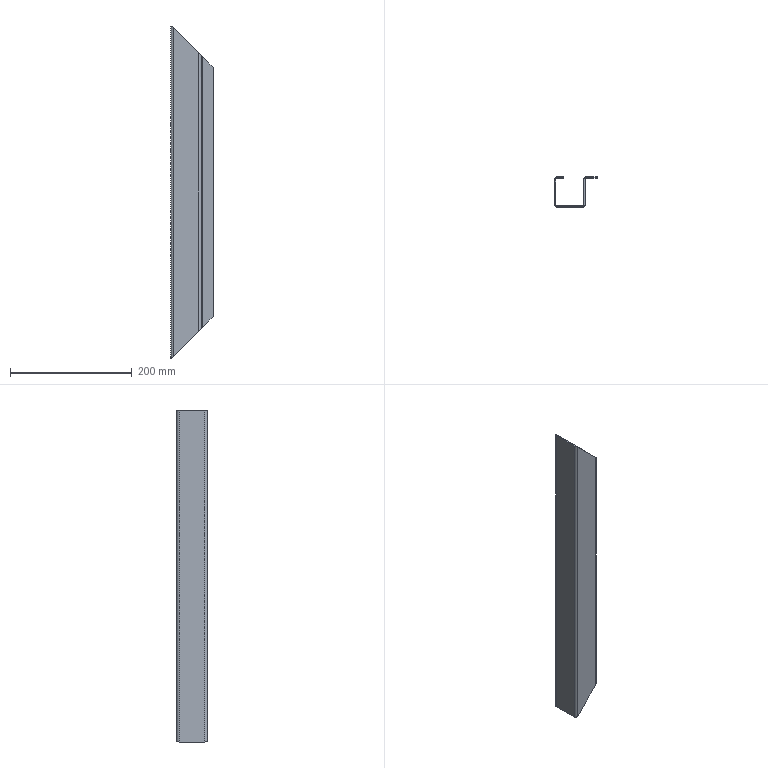Part | STEP file | 750038492 | 1 solid | 38 faces | box 70 x 50 x 546 mm | volume 171514 mm3 | plane 22 | cylinder 8 | spline 8 | commonest cylinder face diameters 4 x4 8 x4
STEP:
#1=CARTESIAN_POINT('',(0.,46.,-273.));
#2=VERTEX_POINT('',#1);
#3=CARTESIAN_POINT('',(0.,4.,-273.));
#4=VERTEX_POINT('',#3);
#5=CARTESIAN_POINT('',(0.,0.,-273.));
#6=DIRECTION('',(0.,-1.,0.));
#7=VECTOR('',#6,1000.);
#8=LINE('',#5,#7);
#9=EDGE_CURVE('',#2,#4,#8,.T.);
#10=ORIENTED_EDGE('',*,*,#9,.T.);
#11=CARTESIAN_POINT('',(0.,4.,273.));
#12=VERTEX_POINT('',#11);
#13=CARTESIAN_POINT('',(0.,4.,275.));
#14=DIRECTION('',(0.,0.,1.));
#15=VECTOR('',#14,1000.);
#16=LINE('',#13,#15);
#17=EDGE_CURVE('',#4,#12,#16,.T.);
#18=ORIENTED_EDGE('',*,*,#17,.T.);
#19=CARTESIAN_POINT('',(0.,46.,273.));
#20=VERTEX_POINT('',#19);
#21=CARTESIAN_POINT('',(0.,0.,273.));
#22=DIRECTION('',(0.,1.,0.));
#23=VECTOR('',#22,1000.);
#24=LINE('',#21,#23);
#25=EDGE_CURVE('',#12,#20,#24,.T.);
#26=ORIENTED_EDGE('',*,*,#25,.T.);
#27=CARTESIAN_POINT('',(0.,46.,275.));
#28=DIRECTION('',(0.,0.,-1.));
#29=VECTOR('',#28,1000.);
#30=LINE('',#27,#29);
#31=EDGE_CURVE('',#20,#2,#30,.T.);
#32=ORIENTED_EDGE('',*,*,#31,.T.);
#33=EDGE_LOOP('',(#10,#18,#26,#32));
#34=FACE_OUTER_BOUND('',#33,.T.);
#35=CARTESIAN_POINT('',(0.,0.,275.));
#36=DIRECTION('',(-1.,0.,0.));
#37=DIRECTION('',(0.,-1.,0.));
#38=AXIS2_PLACEMENT_3D('',#35,#36,#37);
#39=PLANE('',#38);
#40=ADVANCED_FACE('',(#34),#39,.T.);
#41=CARTESIAN_POINT('',(4.,0.,-271.));
#42=VERTEX_POINT('',#41);
#43=CARTESIAN_POINT('',(0.,4.,-273.));
#44=CARTESIAN_POINT('',(0.,2.,-273.));
#45=CARTESIAN_POINT('',(1.333,0.,-272.333));
#46=CARTESIAN_POINT('',(4.,0.,-271.));
#47=(BOUNDED_CURVE()B_SPLINE_CURVE(3,(#43,#44,#45,#46),.UNSPECIFIED.,.F.,.F.)B_SPLINE_CURVE_WITH_KNOTS((4,4),(0.,0.006692),.UNSPECIFIED.)CURVE()GEOMETRIC_REPRESENTATION_ITEM()RATIONAL_B_SPLINE_CURVE((1.,0.6667,0.5,0.5))REPRESENTATION_ITEM(''));
#48=EDGE_CURVE('',#4,#42,#47,.T.);
#49=ORIENTED_EDGE('',*,*,#48,.T.);
#50=CARTESIAN_POINT('',(4.,0.,271.));
#51=VERTEX_POINT('',#50);
#52=CARTESIAN_POINT('',(4.,0.,275.));
#53=DIRECTION('',(0.,0.,1.));
#54=VECTOR('',#53,1000.);
#55=LINE('',#52,#54);
#56=EDGE_CURVE('',#42,#51,#55,.T.);
#57=ORIENTED_EDGE('',*,*,#56,.T.);
#58=CARTESIAN_POINT('',(4.,0.,271.));
#59=CARTESIAN_POINT('',(1.333,0.,272.333));
#60=CARTESIAN_POINT('',(0.,2.,273.));
#61=CARTESIAN_POINT('',(0.,4.,273.));
#62=(BOUNDED_CURVE()B_SPLINE_CURVE(3,(#58,#59,#60,#61),.UNSPECIFIED.,.F.,.F.)B_SPLINE_CURVE_WITH_KNOTS((4,4),(0.,0.006641),.UNSPECIFIED.)CURVE()GEOMETRIC_REPRESENTATION_ITEM()RATIONAL_B_SPLINE_CURVE((0.5,0.5,0.6667,1.))REPRESENTATION_ITEM(''));
#63=EDGE_CURVE('',#51,#12,#62,.T.);
#64=ORIENTED_EDGE('',*,*,#63,.T.);
#65=ORIENTED_EDGE('',*,*,#17,.F.);
#66=EDGE_LOOP('',(#49,#57,#64,#65));
#67=FACE_OUTER_BOUND('',#66,.T.);
#68=CARTESIAN_POINT('',(4.,4.,275.));
#69=DIRECTION('',(0.,0.,-1.));
#70=DIRECTION('',(-1.,0.,0.));
#71=AXIS2_PLACEMENT_3D('',#68,#69,#70);
#72=CYLINDRICAL_SURFACE('',#71,4.);
#73=ADVANCED_FACE('',(#67),#72,.T.);
#74=CARTESIAN_POINT('',(2.,46.,-273.));
#75=VERTEX_POINT('',#74);
#76=CARTESIAN_POINT('',(2.,46.,-273.));
#77=DIRECTION('',(-1.,0.,0.));
#78=VECTOR('',#77,1000.);
#79=LINE('',#76,#78);
#80=EDGE_CURVE('',#75,#2,#79,.T.);
#81=ORIENTED_EDGE('',*,*,#80,.F.);
#82=CARTESIAN_POINT('',(2.,4.,-273.));
#83=VERTEX_POINT('',#82);
#84=CARTESIAN_POINT('',(2.,0.,-273.));
#85=DIRECTION('',(0.,1.,0.));
#86=VECTOR('',#85,1000.);
#87=LINE('',#84,#86);
#88=EDGE_CURVE('',#83,#75,#87,.T.);
#89=ORIENTED_EDGE('',*,*,#88,.F.);
#90=CARTESIAN_POINT('',(2.,4.,-273.));
#91=DIRECTION('',(1.,0.,0.));
#92=VECTOR('',#91,1000.);
#93=LINE('',#90,#92);
#94=EDGE_CURVE('',#4,#83,#93,.T.);
#95=ORIENTED_EDGE('',*,*,#94,.F.);
#96=ORIENTED_EDGE('',*,*,#9,.F.);
#97=EDGE_LOOP('',(#81,#89,#95,#96));
#98=FACE_OUTER_BOUND('',#97,.T.);
#99=CARTESIAN_POINT('',(2.,0.,-273.));
#100=DIRECTION('',(0.,0.,1.));
#101=DIRECTION('',(0.,-1.,0.));
#102=AXIS2_PLACEMENT_3D('',#99,#100,#101);
#103=PLANE('',#102);
#104=ADVANCED_FACE('',(#98),#103,.F.);
#105=CARTESIAN_POINT('',(4.,50.,-271.));
#106=VERTEX_POINT('',#105);
#107=CARTESIAN_POINT('',(4.,50.,-271.));
#108=CARTESIAN_POINT('',(1.333,50.,-272.333));
#109=CARTESIAN_POINT('',(0.,48.,-273.));
#110=CARTESIAN_POINT('',(0.,46.,-273.));
#111=(BOUNDED_CURVE()B_SPLINE_CURVE(3,(#107,#108,#109,#110),.UNSPECIFIED.,.F.,.F.)B_SPLINE_CURVE_WITH_KNOTS((4,4),(0.,0.006641),.UNSPECIFIED.)CURVE()GEOMETRIC_REPRESENTATION_ITEM()RATIONAL_B_SPLINE_CURVE((0.5,0.5,0.6667,1.))REPRESENTATION_ITEM(''));
#112=EDGE_CURVE('',#106,#2,#111,.T.);
#113=ORIENTED_EDGE('',*,*,#112,.T.);
#114=ORIENTED_EDGE('',*,*,#31,.F.);
#115=CARTESIAN_POINT('',(4.,50.,271.));
#116=VERTEX_POINT('',#115);
#117=CARTESIAN_POINT('',(0.,46.,273.));
#118=CARTESIAN_POINT('',(0.,48.,273.));
#119=CARTESIAN_POINT('',(1.333,50.,272.333));
#120=CARTESIAN_POINT('',(4.,50.,271.));
#121=(BOUNDED_CURVE()B_SPLINE_CURVE(3,(#117,#118,#119,#120),.UNSPECIFIED.,.F.,.F.)B_SPLINE_CURVE_WITH_KNOTS((4,4),(0.,0.006627),.UNSPECIFIED.)CURVE()GEOMETRIC_REPRESENTATION_ITEM()RATIONAL_B_SPLINE_CURVE((1.,0.6667,0.5,0.5))REPRESENTATION_ITEM(''));
#122=EDGE_CURVE('',#20,#116,#121,.T.);
#123=ORIENTED_EDGE('',*,*,#122,.T.);
#124=CARTESIAN_POINT('',(4.,50.,275.));
#125=DIRECTION('',(0.,0.,-1.));
#126=VECTOR('',#125,1000.);
#127=LINE('',#124,#126);
#128=EDGE_CURVE('',#116,#106,#127,.T.);
#129=ORIENTED_EDGE('',*,*,#128,.T.);
#130=EDGE_LOOP('',(#113,#114,#123,#129));
#131=FACE_OUTER_BOUND('',#130,.T.);
#132=CARTESIAN_POINT('',(4.,46.,275.));
#133=DIRECTION('',(0.,0.,-1.));
#134=DIRECTION('',(-1.,0.,0.));
#135=AXIS2_PLACEMENT_3D('',#132,#133,#134);
#136=CYLINDRICAL_SURFACE('',#135,4.);
#137=ADVANCED_FACE('',(#131),#136,.T.);
#138=CARTESIAN_POINT('',(2.,46.,273.));
#139=VERTEX_POINT('',#138);
#140=CARTESIAN_POINT('',(2.,4.,273.));
#141=VERTEX_POINT('',#140);
#142=CARTESIAN_POINT('',(2.,0.,273.));
#143=DIRECTION('',(0.,-1.,0.));
#144=VECTOR('',#143,1000.);
#145=LINE('',#142,#144);
#146=EDGE_CURVE('',#139,#141,#145,.T.);
#147=ORIENTED_EDGE('',*,*,#146,.F.);
#148=CARTESIAN_POINT('',(2.,46.,273.));
#149=DIRECTION('',(1.,0.,0.));
#150=VECTOR('',#149,1000.);
#151=LINE('',#148,#150);
#152=EDGE_CURVE('',#20,#139,#151,.T.);
#153=ORIENTED_EDGE('',*,*,#152,.F.);
#154=ORIENTED_EDGE('',*,*,#25,.F.);
#155=CARTESIAN_POINT('',(2.,4.,273.));
#156=DIRECTION('',(-1.,0.,0.));
#157=VECTOR('',#156,1000.);
#158=LINE('',#155,#157);
#159=EDGE_CURVE('',#141,#12,#158,.T.);
#160=ORIENTED_EDGE('',*,*,#159,.F.);
#161=EDGE_LOOP('',(#147,#153,#154,#160));
#162=FACE_OUTER_BOUND('',#161,.T.);
#163=CARTESIAN_POINT('',(2.,0.,273.));
#164=DIRECTION('',(0.,0.,-1.));
#165=DIRECTION('',(0.,1.,0.));
#166=AXIS2_PLACEMENT_3D('',#163,#164,#165);
#167=PLANE('',#166);
#168=ADVANCED_FACE('',(#162),#167,.F.);
#169=CARTESIAN_POINT('',(46.,0.,-229.));
#170=VERTEX_POINT('',#169);
#171=CARTESIAN_POINT('',(4.,0.,-271.));
#172=DIRECTION('',(0.7071,0.,0.7071));
#173=VECTOR('',#172,1000.);
#174=LINE('',#171,#173);
#175=EDGE_CURVE('',#42,#170,#174,.T.);
#176=ORIENTED_EDGE('',*,*,#175,.T.);
#177=CARTESIAN_POINT('',(46.,0.,229.));
#178=VERTEX_POINT('',#177);
#179=CARTESIAN_POINT('',(46.,0.,275.));
#180=DIRECTION('',(0.,0.,1.));
#181=VECTOR('',#180,1000.);
#182=LINE('',#179,#181);
#183=EDGE_CURVE('',#170,#178,#182,.T.);
#184=ORIENTED_EDGE('',*,*,#183,.T.);
#185=CARTESIAN_POINT('',(46.,0.,229.));
#186=DIRECTION('',(-0.7071,0.,0.7071));
#187=VECTOR('',#186,1000.);
#188=LINE('',#185,#187);
#189=EDGE_CURVE('',#178,#51,#188,.T.);
#190=ORIENTED_EDGE('',*,*,#189,.T.);
#191=ORIENTED_EDGE('',*,*,#56,.F.);
#192=EDGE_LOOP('',(#176,#184,#190,#191));
#193=FACE_OUTER_BOUND('',#192,.T.);
#194=CARTESIAN_POINT('',(50.,0.,275.));
#195=DIRECTION('',(0.,-1.,0.));
#196=DIRECTION('',(0.,0.,-1.));
#197=AXIS2_PLACEMENT_3D('',#194,#195,#196);
#198=PLANE('',#197);
#199=ADVANCED_FACE('',(#193),#198,.T.);
#200=CARTESIAN_POINT('',(4.,2.,-271.));
#201=VERTEX_POINT('',#200);
#202=CARTESIAN_POINT('',(4.,1.,-271.));
#203=DIRECTION('',(0.,-1.,0.));
#204=VECTOR('',#203,1000.);
#205=LINE('',#202,#204);
#206=EDGE_CURVE('',#201,#42,#205,.T.);
#207=ORIENTED_EDGE('',*,*,#206,.T.);
#208=ORIENTED_EDGE('',*,*,#48,.F.);
#209=ORIENTED_EDGE('',*,*,#94,.T.);
#210=CARTESIAN_POINT('',(2.,4.,-273.));
#211=CARTESIAN_POINT('',(2.,3.,-273.));
#212=CARTESIAN_POINT('',(2.667,2.,-272.333));
#213=CARTESIAN_POINT('',(4.,2.,-271.));
#214=(BOUNDED_CURVE()B_SPLINE_CURVE(3,(#210,#211,#212,#213),.UNSPECIFIED.,.F.,.F.)B_SPLINE_CURVE_WITH_KNOTS((4,4),(0.,0.003854),.UNSPECIFIED.)CURVE()GEOMETRIC_REPRESENTATION_ITEM()RATIONAL_B_SPLINE_CURVE((1.,0.6667,0.5,0.5))REPRESENTATION_ITEM(''));
#215=EDGE_CURVE('',#83,#201,#214,.T.);
#216=ORIENTED_EDGE('',*,*,#215,.T.);
#217=EDGE_LOOP('',(#207,#208,#209,#216));
#218=FACE_OUTER_BOUND('',#217,.T.);
#219=CARTESIAN_POINT('',(0.,4.,-273.));
#220=CARTESIAN_POINT('',(0.6667,4.,-273.));
#221=CARTESIAN_POINT('',(1.333,4.,-273.));
#222=CARTESIAN_POINT('',(2.,4.,-273.));
#223=CARTESIAN_POINT('',(0.,12.,-273.));
#224=CARTESIAN_POINT('',(0.6667,10.667,-273.));
#225=CARTESIAN_POINT('',(1.333,9.333,-273.));
#226=CARTESIAN_POINT('',(2.,8.,-273.));
#227=CARTESIAN_POINT('',(8.,12.,-269.));
#228=CARTESIAN_POINT('',(7.333,10.667,-269.));
#229=CARTESIAN_POINT('',(6.667,9.333,-269.));
#230=CARTESIAN_POINT('',(6.,8.,-269.));
#231=CARTESIAN_POINT('',(8.,4.,-269.));
#232=CARTESIAN_POINT('',(7.333,4.,-269.));
#233=CARTESIAN_POINT('',(6.667,4.,-269.));
#234=CARTESIAN_POINT('',(6.,4.,-269.));
#235=CARTESIAN_POINT('',(8.,-4.,-269.));
#236=CARTESIAN_POINT('',(7.333,-2.667,-269.));
#237=CARTESIAN_POINT('',(6.667,-1.333,-269.));
#238=CARTESIAN_POINT('',(6.,0.,-269.));
#239=CARTESIAN_POINT('',(0.,-4.,-273.));
#240=CARTESIAN_POINT('',(0.6667,-2.667,-273.));
#241=CARTESIAN_POINT('',(1.333,-1.333,-273.));
#242=CARTESIAN_POINT('',(2.,0.,-273.));
#243=CARTESIAN_POINT('',(0.,4.,-273.));
#244=CARTESIAN_POINT('',(0.6667,4.,-273.));
#245=CARTESIAN_POINT('',(1.333,4.,-273.));
#246=CARTESIAN_POINT('',(2.,4.,-273.));
#247=(BOUNDED_SURFACE()B_SPLINE_SURFACE(3,3,((#219,#220,#221,#222),(#223,#224,#225,#226),(#227,#228,#229,#230),(#231,#232,#233,#234),(#235,#236,#237,#238),(#239,#240,#241,#242),(#243,#244,#245,#246)),.UNSPECIFIED.,.T.,.F.,.F.)B_SPLINE_SURFACE_WITH_KNOTS((4,3,4),(4,4),(0.,0.5,1.),(0.,1.),.UNSPECIFIED.)GEOMETRIC_REPRESENTATION_ITEM()RATIONAL_B_SPLINE_SURFACE(((1.,1.,1.,1.),(0.3333,0.3333,0.3333,0.3333),(0.3333,0.3333,0.3333,0.3333),(1.,1.,1.,1.),(0.3333,0.3333,0.3333,0.3333),(0.3333,0.3333,0.3333,0.3333),(1.,1.,1.,1.)))REPRESENTATION_ITEM('')SURFACE());
#248=ADVANCED_FACE('',(#218),#247,.T.);
#249=ORIENTED_EDGE('',*,*,#159,.T.);
#250=ORIENTED_EDGE('',*,*,#63,.F.);
#251=CARTESIAN_POINT('',(4.,2.,271.));
#252=VERTEX_POINT('',#251);
#253=CARTESIAN_POINT('',(4.,1.,271.));
#254=DIRECTION('',(0.,1.,0.));
#255=VECTOR('',#254,1000.);
#256=LINE('',#253,#255);
#257=EDGE_CURVE('',#51,#252,#256,.T.);
#258=ORIENTED_EDGE('',*,*,#257,.T.);
#259=CARTESIAN_POINT('',(4.,2.,271.));
#260=CARTESIAN_POINT('',(2.667,2.,272.333));
#261=CARTESIAN_POINT('',(2.,3.,273.));
#262=CARTESIAN_POINT('',(2.,4.,273.));
#263=(BOUNDED_CURVE()B_SPLINE_CURVE(3,(#259,#260,#261,#262),.UNSPECIFIED.,.F.,.F.)B_SPLINE_CURVE_WITH_KNOTS((4,4),(0.,0.003785),.UNSPECIFIED.)CURVE()GEOMETRIC_REPRESENTATION_ITEM()RATIONAL_B_SPLINE_CURVE((0.5,0.5,0.6667,1.))REPRESENTATION_ITEM(''));
#264=EDGE_CURVE('',#252,#141,#263,.T.);
#265=ORIENTED_EDGE('',*,*,#264,.T.);
#266=EDGE_LOOP('',(#249,#250,#258,#265));
#267=FACE_OUTER_BOUND('',#266,.T.);
#268=CARTESIAN_POINT('',(8.,4.,269.));
#269=CARTESIAN_POINT('',(7.333,4.,269.));
#270=CARTESIAN_POINT('',(6.667,4.,269.));
#271=CARTESIAN_POINT('',(6.,4.,269.));
#272=CARTESIAN_POINT('',(8.,12.,269.));
#273=CARTESIAN_POINT('',(7.333,10.667,269.));
#274=CARTESIAN_POINT('',(6.667,9.333,269.));
#275=CARTESIAN_POINT('',(6.,8.,269.));
#276=CARTESIAN_POINT('',(0.,12.,273.));
#277=CARTESIAN_POINT('',(0.6667,10.667,273.));
#278=CARTESIAN_POINT('',(1.333,9.333,273.));
#279=CARTESIAN_POINT('',(2.,8.,273.));
#280=CARTESIAN_POINT('',(0.,4.,273.));
#281=CARTESIAN_POINT('',(0.6667,4.,273.));
#282=CARTESIAN_POINT('',(1.333,4.,273.));
#283=CARTESIAN_POINT('',(2.,4.,273.));
#284=CARTESIAN_POINT('',(0.,-4.,273.));
#285=CARTESIAN_POINT('',(0.6667,-2.667,273.));
#286=CARTESIAN_POINT('',(1.333,-1.333,273.));
#287=CARTESIAN_POINT('',(2.,0.,273.));
#288=CARTESIAN_POINT('',(8.,-4.,269.));
#289=CARTESIAN_POINT('',(7.333,-2.667,269.));
#290=CARTESIAN_POINT('',(6.667,-1.333,269.));
#291=CARTESIAN_POINT('',(6.,0.,269.));
#292=CARTESIAN_POINT('',(8.,4.,269.));
#293=CARTESIAN_POINT('',(7.333,4.,269.));
#294=CARTESIAN_POINT('',(6.667,4.,269.));
#295=CARTESIAN_POINT('',(6.,4.,269.));
#296=(BOUNDED_SURFACE()B_SPLINE_SURFACE(3,3,((#268,#269,#270,#271),(#272,#273,#274,#275),(#276,#277,#278,#279),(#280,#281,#282,#283),(#284,#285,#286,#287),(#288,#289,#290,#291),(#292,#293,#294,#295)),.UNSPECIFIED.,.T.,.F.,.F.)B_SPLINE_SURFACE_WITH_KNOTS((4,3,4),(4,4),(0.,0.5,1.),(0.,1.),.UNSPECIFIED.)GEOMETRIC_REPRESENTATION_ITEM()RATIONAL_B_SPLINE_SURFACE(((1.,1.,1.,1.),(0.3333,0.3333,0.3333,0.3333),(0.3333,0.3333,0.3333,0.3333),(1.,1.,1.,1.),(0.3333,0.3333,0.3333,0.3333),(0.3333,0.3333,0.3333,0.3333),(1.,1.,1.,1.)))REPRESENTATION_ITEM('')SURFACE());
#297=ADVANCED_FACE('',(#267),#296,.T.);
#298=ORIENTED_EDGE('',*,*,#80,.T.);
#299=ORIENTED_EDGE('',*,*,#112,.F.);
#300=CARTESIAN_POINT('',(4.,48.,-271.));
#301=VERTEX_POINT('',#300);
#302=CARTESIAN_POINT('',(4.,49.,-271.));
#303=DIRECTION('',(0.,-1.,0.));
#304=VECTOR('',#303,1000.);
#305=LINE('',#302,#304);
#306=EDGE_CURVE('',#106,#301,#305,.T.);
#307=ORIENTED_EDGE('',*,*,#306,.T.);
#308=CARTESIAN_POINT('',(4.,48.,-271.));
#309=CARTESIAN_POINT('',(2.667,48.,-272.333));
#310=CARTESIAN_POINT('',(2.,47.,-273.));
#311=CARTESIAN_POINT('',(2.,46.,-273.));
#312=(BOUNDED_CURVE()B_SPLINE_CURVE(3,(#308,#309,#310,#311),.UNSPECIFIED.,.F.,.F.)B_SPLINE_CURVE_WITH_KNOTS((4,4),(0.,0.003785),.UNSPECIFIED.)CURVE()GEOMETRIC_REPRESENTATION_ITEM()RATIONAL_B_SPLINE_CURVE((0.5,0.5,0.6667,1.))REPRESENTATION_ITEM(''));
#313=EDGE_CURVE('',#301,#75,#312,.T.);
#314=ORIENTED_EDGE('',*,*,#313,.T.);
#315=EDGE_LOOP('',(#298,#299,#307,#314));
#316=FACE_OUTER_BOUND('',#315,.T.);
#317=CARTESIAN_POINT('',(0.,46.,-273.));
#318=CARTESIAN_POINT('',(0.6667,46.,-273.));
#319=CARTESIAN_POINT('',(1.333,46.,-273.));
#320=CARTESIAN_POINT('',(2.,46.,-273.));
#321=CARTESIAN_POINT('',(0.,54.,-273.));
#322=CARTESIAN_POINT('',(0.6667,52.667,-273.));
#323=CARTESIAN_POINT('',(1.333,51.333,-273.));
#324=CARTESIAN_POINT('',(2.,50.,-273.));
#325=CARTESIAN_POINT('',(8.,54.,-269.));
#326=CARTESIAN_POINT('',(7.333,52.667,-269.));
#327=CARTESIAN_POINT('',(6.667,51.333,-269.));
#328=CARTESIAN_POINT('',(6.,50.,-269.));
#329=CARTESIAN_POINT('',(8.,46.,-269.));
#330=CARTESIAN_POINT('',(7.333,46.,-269.));
#331=CARTESIAN_POINT('',(6.667,46.,-269.));
#332=CARTESIAN_POINT('',(6.,46.,-269.));
#333=CARTESIAN_POINT('',(8.,38.,-269.));
#334=CARTESIAN_POINT('',(7.333,39.333,-269.));
#335=CARTESIAN_POINT('',(6.667,40.667,-269.));
#336=CARTESIAN_POINT('',(6.,42.,-269.));
#337=CARTESIAN_POINT('',(0.,38.,-273.));
#338=CARTESIAN_POINT('',(0.6667,39.333,-273.));
#339=CARTESIAN_POINT('',(1.333,40.667,-273.));
#340=CARTESIAN_POINT('',(2.,42.,-273.));
#341=CARTESIAN_POINT('',(0.,46.,-273.));
#342=CARTESIAN_POINT('',(0.6667,46.,-273.));
#343=CARTESIAN_POINT('',(1.333,46.,-273.));
#344=CARTESIAN_POINT('',(2.,46.,-273.));
#345=(BOUNDED_SURFACE()B_SPLINE_SURFACE(3,3,((#317,#318,#319,#320),(#321,#322,#323,#324),(#325,#326,#327,#328),(#329,#330,#331,#332),(#333,#334,#335,#336),(#337,#338,#339,#340),(#341,#342,#343,#344)),.UNSPECIFIED.,.T.,.F.,.F.)B_SPLINE_SURFACE_WITH_KNOTS((4,3,4),(4,4),(0.,0.5,1.),(0.,1.),.UNSPECIFIED.)GEOMETRIC_REPRESENTATION_ITEM()RATIONAL_B_SPLINE_SURFACE(((1.,1.,1.,1.),(0.3333,0.3333,0.3333,0.3333),(0.3333,0.3333,0.3333,0.3333),(1.,1.,1.,1.),(0.3333,0.3333,0.3333,0.3333),(0.3333,0.3333,0.3333,0.3333),(1.,1.,1.,1.)))REPRESENTATION_ITEM('')SURFACE());
#346=ADVANCED_FACE('',(#316),#345,.T.);
#347=ORIENTED_EDGE('',*,*,#146,.T.);
#348=CARTESIAN_POINT('',(2.,4.,275.));
#349=DIRECTION('',(0.,0.,1.));
#350=VECTOR('',#349,1000.);
#351=LINE('',#348,#350);
#352=EDGE_CURVE('',#83,#141,#351,.T.);
#353=ORIENTED_EDGE('',*,*,#352,.F.);
#354=ORIENTED_EDGE('',*,*,#88,.T.);
#355=CARTESIAN_POINT('',(2.,46.,275.));
#356=DIRECTION('',(0.,0.,-1.));
#357=VECTOR('',#356,1000.);
#358=LINE('',#355,#357);
#359=EDGE_CURVE('',#139,#75,#358,.T.);
#360=ORIENTED_EDGE('',*,*,#359,.F.);
#361=EDGE_LOOP('',(#347,#353,#354,#360));
#362=FACE_OUTER_BOUND('',#361,.T.);
#363=CARTESIAN_POINT('',(2.,0.,275.));
#364=DIRECTION('',(-1.,0.,0.));
#365=DIRECTION('',(0.,-1.,0.));
#366=AXIS2_PLACEMENT_3D('',#363,#364,#365);
#367=PLANE('',#366);
#368=ADVANCED_FACE('',(#362),#367,.F.);
#369=CARTESIAN_POINT('',(15.,50.,-260.));
#370=VERTEX_POINT('',#369);
#371=CARTESIAN_POINT('',(15.,50.,-260.));
#372=DIRECTION('',(-0.7071,0.,-0.7071));
#373=VECTOR('',#372,1000.);
#374=LINE('',#371,#373);
#375=EDGE_CURVE('',#370,#106,#374,.T.);
#376=ORIENTED_EDGE('',*,*,#375,.T.);
#377=ORIENTED_EDGE('',*,*,#128,.F.);
#378=CARTESIAN_POINT('',(15.,50.,260.));
#379=VERTEX_POINT('',#378);
#380=CARTESIAN_POINT('',(4.,50.,271.));
#381=DIRECTION('',(0.7071,0.,-0.7071));
#382=VECTOR('',#381,1000.);
#383=LINE('',#380,#382);
#384=EDGE_CURVE('',#116,#379,#383,.T.);
#385=ORIENTED_EDGE('',*,*,#384,.T.);
#386=CARTESIAN_POINT('',(15.,50.,275.));
#387=DIRECTION('',(0.,0.,-1.));
#388=VECTOR('',#387,1000.);
#389=LINE('',#386,#388);
#390=EDGE_CURVE('',#379,#370,#389,.T.);
#391=ORIENTED_EDGE('',*,*,#390,.T.);
#392=EDGE_LOOP('',(#376,#377,#385,#391));
#393=FACE_OUTER_BOUND('',#392,.T.);
#394=CARTESIAN_POINT('',(0.,50.,275.));
#395=DIRECTION('',(0.,1.,0.));
#396=DIRECTION('',(0.,0.,1.));
#397=AXIS2_PLACEMENT_3D('',#394,#395,#396);
#398=PLANE('',#397);
#399=ADVANCED_FACE('',(#393),#398,.T.);
#400=CARTESIAN_POINT('',(4.,48.,271.));
#401=VERTEX_POINT('',#400);
#402=CARTESIAN_POINT('',(4.,49.,271.));
#403=DIRECTION('',(0.,1.,0.));
#404=VECTOR('',#403,1000.);
#405=LINE('',#402,#404);
#406=EDGE_CURVE('',#401,#116,#405,.T.);
#407=ORIENTED_EDGE('',*,*,#406,.T.);
#408=ORIENTED_EDGE('',*,*,#122,.F.);
#409=ORIENTED_EDGE('',*,*,#152,.T.);
#410=CARTESIAN_POINT('',(2.,46.,273.));
#411=CARTESIAN_POINT('',(2.,47.,273.));
#412=CARTESIAN_POINT('',(2.667,48.,272.333));
#413=CARTESIAN_POINT('',(4.,48.,271.));
#414=(BOUNDED_CURVE()B_SPLINE_CURVE(3,(#410,#411,#412,#413),.UNSPECIFIED.,.F.,.F.)B_SPLINE_CURVE_WITH_KNOTS((4,4),(0.,0.003806),.UNSPECIFIED.)CURVE()GEOMETRIC_REPRESENTATION_ITEM()RATIONAL_B_SPLINE_CURVE((1.,0.6667,0.5,0.5))REPRESENTATION_ITEM(''));
#415=EDGE_CURVE('',#139,#401,#414,.T.);
#416=ORIENTED_EDGE('',*,*,#415,.T.);
#417=EDGE_LOOP('',(#407,#408,#409,#416));
#418=FACE_OUTER_BOUND('',#417,.T.);
#419=CARTESIAN_POINT('',(8.,46.,269.));
#420=CARTESIAN_POINT('',(7.333,46.,269.));
#421=CARTESIAN_POINT('',(6.667,46.,269.));
#422=CARTESIAN_POINT('',(6.,46.,269.));
#423=CARTESIAN_POINT('',(8.,54.,269.));
#424=CARTESIAN_POINT('',(7.333,52.667,269.));
#425=CARTESIAN_POINT('',(6.667,51.333,269.));
#426=CARTESIAN_POINT('',(6.,50.,269.));
#427=CARTESIAN_POINT('',(0.,54.,273.));
#428=CARTESIAN_POINT('',(0.6667,52.667,273.));
#429=CARTESIAN_POINT('',(1.333,51.333,273.));
#430=CARTESIAN_POINT('',(2.,50.,273.));
#431=CARTESIAN_POINT('',(0.,46.,273.));
#432=CARTESIAN_POINT('',(0.6667,46.,273.));
#433=CARTESIAN_POINT('',(1.333,46.,273.));
#434=CARTESIAN_POINT('',(2.,46.,273.));
#435=CARTESIAN_POINT('',(0.,38.,273.));
#436=CARTESIAN_POINT('',(0.6667,39.333,273.));
#437=CARTESIAN_POINT('',(1.333,40.667,273.));
#438=CARTESIAN_POINT('',(2.,42.,273.));
#439=CARTESIAN_POINT('',(8.,38.,269.));
#440=CARTESIAN_POINT('',(7.333,39.333,269.));
#441=CARTESIAN_POINT('',(6.667,40.667,269.));
#442=CARTESIAN_POINT('',(6.,42.,269.));
#443=CARTESIAN_POINT('',(8.,46.,269.));
#444=CARTESIAN_POINT('',(7.333,46.,269.));
#445=CARTESIAN_POINT('',(6.667,46.,269.));
#446=CARTESIAN_POINT('',(6.,46.,269.));
#447=(BOUNDED_SURFACE()B_SPLINE_SURFACE(3,3,((#419,#420,#421,#422),(#423,#424,#425,#426),(#427,#428,#429,#430),(#431,#432,#433,#434),(#435,#436,#437,#438),(#439,#440,#441,#442),(#443,#444,#445,#446)),.UNSPECIFIED.,.T.,.F.,.T.)B_SPLINE_SURFACE_WITH_KNOTS((4,3,4),(4,4),(0.,0.5,1.),(0.,1.),.UNSPECIFIED.)GEOMETRIC_REPRESENTATION_ITEM()RATIONAL_B_SPLINE_SURFACE(((1.,1.,1.,1.),(0.3333,0.3333,0.3333,0.3333),(0.3333,0.3333,0.3333,0.3333),(1.,1.,1.,1.),(0.3333,0.3333,0.3333,0.3333),(0.3333,0.3333,0.3333,0.3333),(1.,1.,1.,1.)))REPRESENTATION_ITEM('')SURFACE());
#448=ADVANCED_FACE('',(#418),#447,.T.);
#449=CARTESIAN_POINT('',(50.,4.,-225.));
#450=VERTEX_POINT('',#449);
#451=CARTESIAN_POINT('',(46.,0.,-229.));
#452=CARTESIAN_POINT('',(48.667,0.,-226.333));
#453=CARTESIAN_POINT('',(50.,2.,-225.));
#454=CARTESIAN_POINT('',(50.,4.,-225.));
#455=(BOUNDED_CURVE()B_SPLINE_CURVE(3,(#451,#452,#453,#454),.UNSPECIFIED.,.F.,.T.)B_SPLINE_CURVE_WITH_KNOTS((4,4),(0.,0.007567),.UNSPECIFIED.)CURVE()GEOMETRIC_REPRESENTATION_ITEM()RATIONAL_B_SPLINE_CURVE((0.5,0.5,0.6667,1.))REPRESENTATION_ITEM(''));
#456=EDGE_CURVE('',#170,#450,#455,.T.);
#457=ORIENTED_EDGE('',*,*,#456,.T.);
#458=CARTESIAN_POINT('',(50.,4.,225.));
#459=VERTEX_POINT('',#458);
#460=CARTESIAN_POINT('',(50.,4.,275.));
#461=DIRECTION('',(0.,0.,1.));
#462=VECTOR('',#461,1000.);
#463=LINE('',#460,#462);
#464=EDGE_CURVE('',#450,#459,#463,.T.);
#465=ORIENTED_EDGE('',*,*,#464,.T.);
#466=CARTESIAN_POINT('',(50.,4.,225.));
#467=CARTESIAN_POINT('',(50.,2.,225.));
#468=CARTESIAN_POINT('',(48.667,0.,226.333));
#469=CARTESIAN_POINT('',(46.,0.,229.));
#470=(BOUNDED_CURVE()B_SPLINE_CURVE(3,(#466,#467,#468,#469),.UNSPECIFIED.,.F.,.T.)B_SPLINE_CURVE_WITH_KNOTS((4,4),(0.,0.007712),.UNSPECIFIED.)CURVE()GEOMETRIC_REPRESENTATION_ITEM()RATIONAL_B_SPLINE_CURVE((1.,0.6667,0.5,0.5))REPRESENTATION_ITEM(''));
#471=EDGE_CURVE('',#459,#178,#470,.T.);
#472=ORIENTED_EDGE('',*,*,#471,.T.);
#473=ORIENTED_EDGE('',*,*,#183,.F.);
#474=EDGE_LOOP('',(#457,#465,#472,#473));
#475=FACE_OUTER_BOUND('',#474,.T.);
#476=CARTESIAN_POINT('',(46.,4.,275.));
#477=DIRECTION('',(0.,0.,-1.));
#478=DIRECTION('',(-1.,0.,0.));
#479=AXIS2_PLACEMENT_3D('',#476,#477,#478);
#480=CYLINDRICAL_SURFACE('',#479,4.);
#481=ADVANCED_FACE('',(#475),#480,.T.);
#482=ORIENTED_EDGE('',*,*,#175,.F.);
#483=ORIENTED_EDGE('',*,*,#206,.F.);
#484=CARTESIAN_POINT('',(46.,2.,-229.));
#485=VERTEX_POINT('',#484);
#486=CARTESIAN_POINT('',(300.,2.,25.));
#487=DIRECTION('',(-0.7071,0.,-0.7071));
#488=VECTOR('',#487,1000.);
#489=LINE('',#486,#488);
#490=EDGE_CURVE('',#485,#201,#489,.T.);
#491=ORIENTED_EDGE('',*,*,#490,.F.);
#492=CARTESIAN_POINT('',(46.,0.,-229.));
#493=DIRECTION('',(0.,1.,0.));
#494=VECTOR('',#493,1000.);
#495=LINE('',#492,#494);
#496=EDGE_CURVE('',#170,#485,#495,.T.);
#497=ORIENTED_EDGE('',*,*,#496,.F.);
#498=EDGE_LOOP('',(#482,#483,#491,#497));
#499=FACE_OUTER_BOUND('',#498,.T.);
#500=CARTESIAN_POINT('',(300.,0.,25.));
#501=DIRECTION('',(-0.7071,0.,0.7071));
#502=DIRECTION('',(0.7071,0.,0.7071));
#503=AXIS2_PLACEMENT_3D('',#500,#501,#502);
#504=PLANE('',#503);
#505=ADVANCED_FACE('',(#499),#504,.F.);
#506=ORIENTED_EDGE('',*,*,#189,.F.);
#507=CARTESIAN_POINT('',(46.,2.,229.));
#508=VERTEX_POINT('',#507);
#509=CARTESIAN_POINT('',(46.,0.,229.));
#510=DIRECTION('',(0.,-1.,0.));
#511=VECTOR('',#510,1000.);
#512=LINE('',#509,#511);
#513=EDGE_CURVE('',#508,#178,#512,.T.);
#514=ORIENTED_EDGE('',*,*,#513,.F.);
#515=CARTESIAN_POINT('',(25.,2.,250.));
#516=DIRECTION('',(0.7071,0.,-0.7071));
#517=VECTOR('',#516,1000.);
#518=LINE('',#515,#517);
#519=EDGE_CURVE('',#252,#508,#518,.T.);
#520=ORIENTED_EDGE('',*,*,#519,.F.);
#521=ORIENTED_EDGE('',*,*,#257,.F.);
#522=EDGE_LOOP('',(#506,#514,#520,#521));
#523=FACE_OUTER_BOUND('',#522,.T.);
#524=CARTESIAN_POINT('',(25.,0.,250.));
#525=DIRECTION('',(-0.7071,0.,-0.7071));
#526=DIRECTION('',(-0.7071,0.,0.7071));
#527=AXIS2_PLACEMENT_3D('',#524,#525,#526);
#528=PLANE('',#527);
#529=ADVANCED_FACE('',(#523),#528,.F.);
#530=ORIENTED_EDGE('',*,*,#264,.F.);
#531=CARTESIAN_POINT('',(4.,2.,275.));
#532=DIRECTION('',(0.,0.,1.));
#533=VECTOR('',#532,1000.);
#534=LINE('',#531,#533);
#535=EDGE_CURVE('',#201,#252,#534,.T.);
#536=ORIENTED_EDGE('',*,*,#535,.F.);
#537=ORIENTED_EDGE('',*,*,#215,.F.);
#538=ORIENTED_EDGE('',*,*,#352,.T.);
#539=EDGE_LOOP('',(#530,#536,#537,#538));
#540=FACE_OUTER_BOUND('',#539,.T.);
#541=CARTESIAN_POINT('',(4.,4.,275.));
#542=DIRECTION('',(0.,0.,-1.));
#543=DIRECTION('',(-1.,0.,0.));
#544=AXIS2_PLACEMENT_3D('',#541,#542,#543);
#545=CYLINDRICAL_SURFACE('',#544,2.);
#546=ADVANCED_FACE('',(#540),#545,.F.);
#547=ORIENTED_EDGE('',*,*,#415,.F.);
#548=ORIENTED_EDGE('',*,*,#359,.T.);
#549=ORIENTED_EDGE('',*,*,#313,.F.);
#550=CARTESIAN_POINT('',(4.,48.,275.));
#551=DIRECTION('',(0.,0.,-1.));
#552=VECTOR('',#551,1000.);
#553=LINE('',#550,#552);
#554=EDGE_CURVE('',#401,#301,#553,.T.);
#555=ORIENTED_EDGE('',*,*,#554,.F.);
#556=EDGE_LOOP('',(#547,#548,#549,#555));
#557=FACE_OUTER_BOUND('',#556,.T.);
#558=CARTESIAN_POINT('',(4.,46.,275.));
#559=DIRECTION('',(0.,0.,-1.));
#560=DIRECTION('',(-1.,0.,0.));
#561=AXIS2_PLACEMENT_3D('',#558,#559,#560);
#562=CYLINDRICAL_SURFACE('',#561,2.);
#563=ADVANCED_FACE('',(#557),#562,.F.);
#564=ORIENTED_EDGE('',*,*,#375,.F.);
#565=CARTESIAN_POINT('',(15.,48.,-260.));
#566=VERTEX_POINT('',#565);
#567=CARTESIAN_POINT('',(15.,50.,-260.));
#568=DIRECTION('',(0.,1.,0.));
#569=VECTOR('',#568,1000.);
#570=LINE('',#567,#569);
#571=EDGE_CURVE('',#566,#370,#570,.T.);
#572=ORIENTED_EDGE('',*,*,#571,.F.);
#573=CARTESIAN_POINT('',(275.,48.,0.));
#574=DIRECTION('',(0.7071,0.,0.7071));
#575=VECTOR('',#574,1000.);
#576=LINE('',#573,#575);
#577=EDGE_CURVE('',#301,#566,#576,.T.);
#578=ORIENTED_EDGE('',*,*,#577,.F.);
#579=ORIENTED_EDGE('',*,*,#306,.F.);
#580=EDGE_LOOP('',(#564,#572,#578,#579));
#581=FACE_OUTER_BOUND('',#580,.T.);
#582=CARTESIAN_POINT('',(275.,50.,0.));
#583=DIRECTION('',(-0.7071,0.,0.7071));
#584=DIRECTION('',(0.7071,0.,0.7071));
#585=AXIS2_PLACEMENT_3D('',#582,#583,#584);
#586=PLANE('',#585);
#587=ADVANCED_FACE('',(#581),#586,.F.);
#588=ORIENTED_EDGE('',*,*,#571,.T.);
#589=ORIENTED_EDGE('',*,*,#390,.F.);
#590=CARTESIAN_POINT('',(15.,48.,260.));
#591=VERTEX_POINT('',#590);
#592=CARTESIAN_POINT('',(15.,50.,260.));
#593=DIRECTION('',(0.,-1.,0.));
#594=VECTOR('',#593,1000.);
#595=LINE('',#592,#594);
#596=EDGE_CURVE('',#379,#591,#595,.T.);
#597=ORIENTED_EDGE('',*,*,#596,.T.);
#598=CARTESIAN_POINT('',(15.,48.,275.));
#599=DIRECTION('',(0.,0.,-1.));
#600=VECTOR('',#599,1000.);
#601=LINE('',#598,#600);
#602=EDGE_CURVE('',#591,#566,#601,.T.);
#603=ORIENTED_EDGE('',*,*,#602,.T.);
#604=EDGE_LOOP('',(#588,#589,#597,#603));
#605=FACE_OUTER_BOUND('',#604,.T.);
#606=CARTESIAN_POINT('',(15.,50.,275.));
#607=DIRECTION('',(1.,0.,0.));
#608=DIRECTION('',(0.,0.,-1.));
#609=AXIS2_PLACEMENT_3D('',#606,#607,#608);
#610=PLANE('',#609);
#611=ADVANCED_FACE('',(#605),#610,.T.);
#612=ORIENTED_EDGE('',*,*,#384,.F.);
#613=ORIENTED_EDGE('',*,*,#406,.F.);
#614=CARTESIAN_POINT('',(0.,48.,275.));
#615=DIRECTION('',(-0.7071,0.,0.7071));
#616=VECTOR('',#615,1000.);
#617=LINE('',#614,#616);
#618=EDGE_CURVE('',#591,#401,#617,.T.);
#619=ORIENTED_EDGE('',*,*,#618,.F.);
#620=ORIENTED_EDGE('',*,*,#596,.F.);
#621=EDGE_LOOP('',(#612,#613,#619,#620));
#622=FACE_OUTER_BOUND('',#621,.T.);
#623=CARTESIAN_POINT('',(0.,50.,275.));
#624=DIRECTION('',(-0.7071,0.,-0.7071));
#625=DIRECTION('',(-0.7071,0.,0.7071));
#626=AXIS2_PLACEMENT_3D('',#623,#624,#625);
#627=PLANE('',#626);
#628=ADVANCED_FACE('',(#622),#627,.F.);
#629=CARTESIAN_POINT('',(50.,46.,-225.));
#630=VERTEX_POINT('',#629);
#631=CARTESIAN_POINT('',(50.,48.,-225.));
#632=DIRECTION('',(0.,1.,0.));
#633=VECTOR('',#632,1000.);
#634=LINE('',#631,#633);
#635=EDGE_CURVE('',#450,#630,#634,.T.);
#636=ORIENTED_EDGE('',*,*,#635,.T.);
#637=CARTESIAN_POINT('',(50.,46.,225.));
#638=VERTEX_POINT('',#637);
#639=CARTESIAN_POINT('',(50.,46.,275.));
#640=DIRECTION('',(0.,0.,1.));
#641=VECTOR('',#640,1000.);
#642=LINE('',#639,#641);
#643=EDGE_CURVE('',#630,#638,#642,.T.);
#644=ORIENTED_EDGE('',*,*,#643,.T.);
#645=CARTESIAN_POINT('',(50.,48.,225.));
#646=DIRECTION('',(0.,-1.,0.));
#647=VECTOR('',#646,1000.);
#648=LINE('',#645,#647);
#649=EDGE_CURVE('',#638,#459,#648,.T.);
#650=ORIENTED_EDGE('',*,*,#649,.T.);
#651=ORIENTED_EDGE('',*,*,#464,.F.);
#652=EDGE_LOOP('',(#636,#644,#650,#651));
#653=FACE_OUTER_BOUND('',#652,.T.);
#654=CARTESIAN_POINT('',(50.,48.,275.));
#655=DIRECTION('',(1.,0.,0.));
#656=DIRECTION('',(0.,1.,0.));
#657=AXIS2_PLACEMENT_3D('',#654,#655,#656);
#658=PLANE('',#657);
#659=ADVANCED_FACE('',(#653),#658,.T.);
#660=ORIENTED_EDGE('',*,*,#496,.T.);
#661=CARTESIAN_POINT('',(48.,4.,-225.));
#662=VERTEX_POINT('',#661);
#663=CARTESIAN_POINT('',(46.,2.,-229.));
#664=CARTESIAN_POINT('',(47.333,2.,-226.333));
#665=CARTESIAN_POINT('',(48.,3.,-225.));
#666=CARTESIAN_POINT('',(48.,4.,-225.));
#667=(BOUNDED_CURVE()B_SPLINE_CURVE(3,(#663,#664,#665,#666),.UNSPECIFIED.,.F.,.F.)B_SPLINE_CURVE_WITH_KNOTS((4,4),(0.,0.005228),.UNSPECIFIED.)CURVE()GEOMETRIC_REPRESENTATION_ITEM()RATIONAL_B_SPLINE_CURVE((0.5,0.5,0.6667,1.))REPRESENTATION_ITEM(''));
#668=EDGE_CURVE('',#485,#662,#667,.T.);
#669=ORIENTED_EDGE('',*,*,#668,.T.);
#670=CARTESIAN_POINT('',(49.,4.,-225.));
#671=DIRECTION('',(1.,0.,0.));
#672=VECTOR('',#671,1000.);
#673=LINE('',#670,#672);
#674=EDGE_CURVE('',#662,#450,#673,.T.);
#675=ORIENTED_EDGE('',*,*,#674,.T.);
#676=ORIENTED_EDGE('',*,*,#456,.F.);
#677=EDGE_LOOP('',(#660,#669,#675,#676));
#678=FACE_OUTER_BOUND('',#677,.T.);
#679=CARTESIAN_POINT('',(42.,4.,-233.));
#680=CARTESIAN_POINT('',(42.667,4.,-233.));
#681=CARTESIAN_POINT('',(43.333,4.,-233.));
#682=CARTESIAN_POINT('',(44.,4.,-233.));
#683=CARTESIAN_POINT('',(42.,12.,-233.));
#684=CARTESIAN_POINT('',(42.667,10.667,-233.));
#685=CARTESIAN_POINT('',(43.333,9.333,-233.));
#686=CARTESIAN_POINT('',(44.,8.,-233.));
#687=CARTESIAN_POINT('',(50.,12.,-225.));
#688=CARTESIAN_POINT('',(49.333,10.667,-225.));
#689=CARTESIAN_POINT('',(48.667,9.333,-225.));
#690=CARTESIAN_POINT('',(48.,8.,-225.));
#691=CARTESIAN_POINT('',(50.,4.,-225.));
#692=CARTESIAN_POINT('',(49.333,4.,-225.));
#693=CARTESIAN_POINT('',(48.667,4.,-225.));
#694=CARTESIAN_POINT('',(48.,4.,-225.));
#695=CARTESIAN_POINT('',(50.,-4.,-225.));
#696=CARTESIAN_POINT('',(49.333,-2.667,-225.));
#697=CARTESIAN_POINT('',(48.667,-1.333,-225.));
#698=CARTESIAN_POINT('',(48.,0.,-225.));
#699=CARTESIAN_POINT('',(42.,-4.,-233.));
#700=CARTESIAN_POINT('',(42.667,-2.667,-233.));
#701=CARTESIAN_POINT('',(43.333,-1.333,-233.));
#702=CARTESIAN_POINT('',(44.,0.,-233.));
#703=CARTESIAN_POINT('',(42.,4.,-233.));
#704=CARTESIAN_POINT('',(42.667,4.,-233.));
#705=CARTESIAN_POINT('',(43.333,4.,-233.));
#706=CARTESIAN_POINT('',(44.,4.,-233.));
#707=(BOUNDED_SURFACE()B_SPLINE_SURFACE(3,3,((#679,#680,#681,#682),(#683,#684,#685,#686),(#687,#688,#689,#690),(#691,#692,#693,#694),(#695,#696,#697,#698),(#699,#700,#701,#702),(#703,#704,#705,#706)),.UNSPECIFIED.,.T.,.F.,.T.)B_SPLINE_SURFACE_WITH_KNOTS((4,3,4),(4,4),(0.,0.5,1.),(0.,1.),.UNSPECIFIED.)GEOMETRIC_REPRESENTATION_ITEM()RATIONAL_B_SPLINE_SURFACE(((1.,1.,1.,1.),(0.3333,0.3333,0.3333,0.3333),(0.3333,0.3333,0.3333,0.3333),(1.,1.,1.,1.),(0.3333,0.3333,0.3333,0.3333),(0.3333,0.3333,0.3333,0.3333),(1.,1.,1.,1.)))REPRESENTATION_ITEM('')SURFACE());
#708=ADVANCED_FACE('',(#678),#707,.T.);
#709=CARTESIAN_POINT('',(48.,4.,225.));
#710=VERTEX_POINT('',#709);
#711=CARTESIAN_POINT('',(49.,4.,225.));
#712=DIRECTION('',(-1.,0.,0.));
#713=VECTOR('',#712,1000.);
#714=LINE('',#711,#713);
#715=EDGE_CURVE('',#459,#710,#714,.T.);
#716=ORIENTED_EDGE('',*,*,#715,.T.);
#717=CARTESIAN_POINT('',(48.,4.,225.));
#718=CARTESIAN_POINT('',(48.,3.,225.));
#719=CARTESIAN_POINT('',(47.333,2.,226.333));
#720=CARTESIAN_POINT('',(46.,2.,229.));
#721=(BOUNDED_CURVE()B_SPLINE_CURVE(3,(#717,#718,#719,#720),.UNSPECIFIED.,.F.,.F.)B_SPLINE_CURVE_WITH_KNOTS((4,4),(0.,0.00529),.UNSPECIFIED.)CURVE()GEOMETRIC_REPRESENTATION_ITEM()RATIONAL_B_SPLINE_CURVE((1.,0.6667,0.5,0.5))REPRESENTATION_ITEM(''));
#722=EDGE_CURVE('',#710,#508,#721,.T.);
#723=ORIENTED_EDGE('',*,*,#722,.T.);
#724=ORIENTED_EDGE('',*,*,#513,.T.);
#725=ORIENTED_EDGE('',*,*,#471,.F.);
#726=EDGE_LOOP('',(#716,#723,#724,#725));
#727=FACE_OUTER_BOUND('',#726,.T.);
#728=CARTESIAN_POINT('',(50.,4.,225.));
#729=CARTESIAN_POINT('',(49.333,4.,225.));
#730=CARTESIAN_POINT('',(48.667,4.,225.));
#731=CARTESIAN_POINT('',(48.,4.,225.));
#732=CARTESIAN_POINT('',(50.,12.,225.));
#733=CARTESIAN_POINT('',(49.333,10.667,225.));
#734=CARTESIAN_POINT('',(48.667,9.333,225.));
#735=CARTESIAN_POINT('',(48.,8.,225.));
#736=CARTESIAN_POINT('',(42.,12.,233.));
#737=CARTESIAN_POINT('',(42.667,10.667,233.));
#738=CARTESIAN_POINT('',(43.333,9.333,233.));
#739=CARTESIAN_POINT('',(44.,8.,233.));
#740=CARTESIAN_POINT('',(42.,4.,233.));
#741=CARTESIAN_POINT('',(42.667,4.,233.));
#742=CARTESIAN_POINT('',(43.333,4.,233.));
#743=CARTESIAN_POINT('',(44.,4.,233.));
#744=CARTESIAN_POINT('',(42.,-4.,233.));
#745=CARTESIAN_POINT('',(42.667,-2.667,233.));
#746=CARTESIAN_POINT('',(43.333,-1.333,233.));
#747=CARTESIAN_POINT('',(44.,0.,233.));
#748=CARTESIAN_POINT('',(50.,-4.,225.));
#749=CARTESIAN_POINT('',(49.333,-2.667,225.));
#750=CARTESIAN_POINT('',(48.667,-1.333,225.));
#751=CARTESIAN_POINT('',(48.,0.,225.));
#752=CARTESIAN_POINT('',(50.,4.,225.));
#753=CARTESIAN_POINT('',(49.333,4.,225.));
#754=CARTESIAN_POINT('',(48.667,4.,225.));
#755=CARTESIAN_POINT('',(48.,4.,225.));
#756=(BOUNDED_SURFACE()B_SPLINE_SURFACE(3,3,((#728,#729,#730,#731),(#732,#733,#734,#735),(#736,#737,#738,#739),(#740,#741,#742,#743),(#744,#745,#746,#747),(#748,#749,#750,#751),(#752,#753,#754,#755)),.UNSPECIFIED.,.T.,.F.,.F.)B_SPLINE_SURFACE_WITH_KNOTS((4,3,4),(4,4),(0.,0.5,1.),(0.,1.),.UNSPECIFIED.)GEOMETRIC_REPRESENTATION_ITEM()RATIONAL_B_SPLINE_SURFACE(((1.,1.,1.,1.),(0.3333,0.3333,0.3333,0.3333),(0.3333,0.3333,0.3333,0.3333),(1.,1.,1.,1.),(0.3333,0.3333,0.3333,0.3333),(0.3333,0.3333,0.3333,0.3333),(1.,1.,1.,1.)))REPRESENTATION_ITEM('')SURFACE());
#757=ADVANCED_FACE('',(#727),#756,.T.);
#758=ORIENTED_EDGE('',*,*,#519,.T.);
#759=CARTESIAN_POINT('',(46.,2.,275.));
#760=DIRECTION('',(0.,0.,1.));
#761=VECTOR('',#760,1000.);
#762=LINE('',#759,#761);
#763=EDGE_CURVE('',#485,#508,#762,.T.);
#764=ORIENTED_EDGE('',*,*,#763,.F.);
#765=ORIENTED_EDGE('',*,*,#490,.T.);
#766=ORIENTED_EDGE('',*,*,#535,.T.);
#767=EDGE_LOOP('',(#758,#764,#765,#766));
#768=FACE_OUTER_BOUND('',#767,.T.);
#769=CARTESIAN_POINT('',(50.,2.,275.));
#770=DIRECTION('',(0.,-1.,0.));
#771=DIRECTION('',(0.,0.,-1.));
#772=AXIS2_PLACEMENT_3D('',#769,#770,#771);
#773=PLANE('',#772);
#774=ADVANCED_FACE('',(#768),#773,.F.);
#775=ORIENTED_EDGE('',*,*,#618,.T.);
#776=ORIENTED_EDGE('',*,*,#554,.T.);
#777=ORIENTED_EDGE('',*,*,#577,.T.);
#778=ORIENTED_EDGE('',*,*,#602,.F.);
#779=EDGE_LOOP('',(#775,#776,#777,#778));
#780=FACE_OUTER_BOUND('',#779,.T.);
#781=CARTESIAN_POINT('',(0.,48.,275.));
#782=DIRECTION('',(0.,1.,0.));
#783=DIRECTION('',(0.,0.,1.));
#784=AXIS2_PLACEMENT_3D('',#781,#782,#783);
#785=PLANE('',#784);
#786=ADVANCED_FACE('',(#780),#785,.F.);
#787=ORIENTED_EDGE('',*,*,#643,.F.);
#788=CARTESIAN_POINT('',(52.,48.,-223.));
#789=VERTEX_POINT('',#788);
#790=CARTESIAN_POINT('',(52.,48.,-223.));
#791=CARTESIAN_POINT('',(50.667,48.,-224.333));
#792=CARTESIAN_POINT('',(50.,47.,-225.));
#793=CARTESIAN_POINT('',(50.,46.,-225.));
#794=(BOUNDED_CURVE()B_SPLINE_CURVE(3,(#790,#791,#792,#793),.UNSPECIFIED.,.F.,.F.)B_SPLINE_CURVE_WITH_KNOTS((4,4),(0.,0.003785),.UNSPECIFIED.)CURVE()GEOMETRIC_REPRESENTATION_ITEM()RATIONAL_B_SPLINE_CURVE((0.5,0.5,0.6667,1.))REPRESENTATION_ITEM(''));
#795=EDGE_CURVE('',#789,#630,#794,.T.);
#796=ORIENTED_EDGE('',*,*,#795,.F.);
#797=CARTESIAN_POINT('',(52.,48.,223.));
#798=VERTEX_POINT('',#797);
#799=CARTESIAN_POINT('',(52.,48.,275.));
#800=DIRECTION('',(0.,0.,-1.));
#801=VECTOR('',#800,1000.);
#802=LINE('',#799,#801);
#803=EDGE_CURVE('',#798,#789,#802,.T.);
#804=ORIENTED_EDGE('',*,*,#803,.F.);
#805=CARTESIAN_POINT('',(50.,46.,225.));
#806=CARTESIAN_POINT('',(50.,47.,225.));
#807=CARTESIAN_POINT('',(50.667,48.,224.333));
#808=CARTESIAN_POINT('',(52.,48.,223.));
#809=(BOUNDED_CURVE()B_SPLINE_CURVE(3,(#805,#806,#807,#808),.UNSPECIFIED.,.F.,.F.)B_SPLINE_CURVE_WITH_KNOTS((4,4),(0.,0.003854),.UNSPECIFIED.)CURVE()GEOMETRIC_REPRESENTATION_ITEM()RATIONAL_B_SPLINE_CURVE((1.,0.6667,0.5,0.5))REPRESENTATION_ITEM(''));
#810=EDGE_CURVE('',#638,#798,#809,.T.);
#811=ORIENTED_EDGE('',*,*,#810,.F.);
#812=EDGE_LOOP('',(#787,#796,#804,#811));
#813=FACE_OUTER_BOUND('',#812,.T.);
#814=CARTESIAN_POINT('',(52.,46.,275.));
#815=DIRECTION('',(0.,0.,-1.));
#816=DIRECTION('',(-1.,0.,0.));
#817=AXIS2_PLACEMENT_3D('',#814,#815,#816);
#818=CYLINDRICAL_SURFACE('',#817,2.);
#819=ADVANCED_FACE('',(#813),#818,.F.);
#820=ORIENTED_EDGE('',*,*,#635,.F.);
#821=ORIENTED_EDGE('',*,*,#674,.F.);
#822=CARTESIAN_POINT('',(48.,46.,-225.));
#823=VERTEX_POINT('',#822);
#824=CARTESIAN_POINT('',(48.,48.,-225.));
#825=DIRECTION('',(0.,-1.,0.));
#826=VECTOR('',#825,1000.);
#827=LINE('',#824,#826);
#828=EDGE_CURVE('',#823,#662,#827,.T.);
#829=ORIENTED_EDGE('',*,*,#828,.F.);
#830=CARTESIAN_POINT('',(50.,46.,-225.));
#831=DIRECTION('',(-1.,0.,0.));
#832=VECTOR('',#831,1000.);
#833=LINE('',#830,#832);
#834=EDGE_CURVE('',#630,#823,#833,.T.);
#835=ORIENTED_EDGE('',*,*,#834,.F.);
#836=EDGE_LOOP('',(#820,#821,#829,#835));
#837=FACE_OUTER_BOUND('',#836,.T.);
#838=CARTESIAN_POINT('',(50.,48.,-225.));
#839=DIRECTION('',(0.,0.,1.));
#840=DIRECTION('',(0.,-1.,0.));
#841=AXIS2_PLACEMENT_3D('',#838,#839,#840);
#842=PLANE('',#841);
#843=ADVANCED_FACE('',(#837),#842,.F.);
#844=ORIENTED_EDGE('',*,*,#649,.F.);
#845=CARTESIAN_POINT('',(48.,46.,225.));
#846=VERTEX_POINT('',#845);
#847=CARTESIAN_POINT('',(50.,46.,225.));
#848=DIRECTION('',(1.,0.,0.));
#849=VECTOR('',#848,1000.);
#850=LINE('',#847,#849);
#851=EDGE_CURVE('',#846,#638,#850,.T.);
#852=ORIENTED_EDGE('',*,*,#851,.F.);
#853=CARTESIAN_POINT('',(48.,48.,225.));
#854=DIRECTION('',(0.,1.,0.));
#855=VECTOR('',#854,1000.);
#856=LINE('',#853,#855);
#857=EDGE_CURVE('',#710,#846,#856,.T.);
#858=ORIENTED_EDGE('',*,*,#857,.F.);
#859=ORIENTED_EDGE('',*,*,#715,.F.);
#860=EDGE_LOOP('',(#844,#852,#858,#859));
#861=FACE_OUTER_BOUND('',#860,.T.);
#862=CARTESIAN_POINT('',(50.,48.,225.));
#863=DIRECTION('',(0.,0.,-1.));
#864=DIRECTION('',(0.,1.,0.));
#865=AXIS2_PLACEMENT_3D('',#862,#863,#864);
#866=PLANE('',#865);
#867=ADVANCED_FACE('',(#861),#866,.F.);
#868=ORIENTED_EDGE('',*,*,#722,.F.);
#869=CARTESIAN_POINT('',(48.,4.,275.));
#870=DIRECTION('',(0.,0.,1.));
#871=VECTOR('',#870,1000.);
#872=LINE('',#869,#871);
#873=EDGE_CURVE('',#662,#710,#872,.T.);
#874=ORIENTED_EDGE('',*,*,#873,.F.);
#875=ORIENTED_EDGE('',*,*,#668,.F.);
#876=ORIENTED_EDGE('',*,*,#763,.T.);
#877=EDGE_LOOP('',(#868,#874,#875,#876));
#878=FACE_OUTER_BOUND('',#877,.T.);
#879=CARTESIAN_POINT('',(46.,4.,275.));
#880=DIRECTION('',(0.,0.,-1.));
#881=DIRECTION('',(-1.,0.,0.));
#882=AXIS2_PLACEMENT_3D('',#879,#880,#881);
#883=CYLINDRICAL_SURFACE('',#882,2.);
#884=ADVANCED_FACE('',(#878),#883,.F.);
#885=CARTESIAN_POINT('',(52.,50.,223.));
#886=VERTEX_POINT('',#885);
#887=CARTESIAN_POINT('',(52.,49.,223.));
#888=DIRECTION('',(0.,1.,0.));
#889=VECTOR('',#888,1000.);
#890=LINE('',#887,#889);
#891=EDGE_CURVE('',#798,#886,#890,.T.);
#892=ORIENTED_EDGE('',*,*,#891,.T.);
#893=CARTESIAN_POINT('',(52.,50.,223.));
#894=CARTESIAN_POINT('',(49.333,50.,224.333));
#895=CARTESIAN_POINT('',(48.,48.,225.));
#896=CARTESIAN_POINT('',(48.,46.,225.));
#897=(BOUNDED_CURVE()B_SPLINE_CURVE(3,(#893,#894,#895,#896),.UNSPECIFIED.,.F.,.F.)B_SPLINE_CURVE_WITH_KNOTS((4,4),(0.,0.006622),.UNSPECIFIED.)CURVE()GEOMETRIC_REPRESENTATION_ITEM()RATIONAL_B_SPLINE_CURVE((0.5,0.5,0.6667,1.))REPRESENTATION_ITEM(''));
#898=EDGE_CURVE('',#886,#846,#897,.T.);
#899=ORIENTED_EDGE('',*,*,#898,.T.);
#900=ORIENTED_EDGE('',*,*,#851,.T.);
#901=ORIENTED_EDGE('',*,*,#810,.T.);
#902=EDGE_LOOP('',(#892,#899,#900,#901));
#903=FACE_OUTER_BOUND('',#902,.T.);
#904=CARTESIAN_POINT('',(54.,46.,221.));
#905=CARTESIAN_POINT('',(54.667,46.,221.));
#906=CARTESIAN_POINT('',(55.333,46.,221.));
#907=CARTESIAN_POINT('',(56.,46.,221.));
#908=CARTESIAN_POINT('',(54.,42.,221.));
#909=CARTESIAN_POINT('',(54.667,40.667,221.));
#910=CARTESIAN_POINT('',(55.333,39.333,221.));
#911=CARTESIAN_POINT('',(56.,38.,221.));
#912=CARTESIAN_POINT('',(50.,42.,225.));
#913=CARTESIAN_POINT('',(49.333,40.667,225.));
#914=CARTESIAN_POINT('',(48.667,39.333,225.));
#915=CARTESIAN_POINT('',(48.,38.,225.));
#916=CARTESIAN_POINT('',(50.,46.,225.));
#917=CARTESIAN_POINT('',(49.333,46.,225.));
#918=CARTESIAN_POINT('',(48.667,46.,225.));
#919=CARTESIAN_POINT('',(48.,46.,225.));
#920=CARTESIAN_POINT('',(50.,50.,225.));
#921=CARTESIAN_POINT('',(49.333,51.333,225.));
#922=CARTESIAN_POINT('',(48.667,52.667,225.));
#923=CARTESIAN_POINT('',(48.,54.,225.));
#924=CARTESIAN_POINT('',(54.,50.,221.));
#925=CARTESIAN_POINT('',(54.667,51.333,221.));
#926=CARTESIAN_POINT('',(55.333,52.667,221.));
#927=CARTESIAN_POINT('',(56.,54.,221.));
#928=CARTESIAN_POINT('',(54.,46.,221.));
#929=CARTESIAN_POINT('',(54.667,46.,221.));
#930=CARTESIAN_POINT('',(55.333,46.,221.));
#931=CARTESIAN_POINT('',(56.,46.,221.));
#932=(BOUNDED_SURFACE()B_SPLINE_SURFACE(3,3,((#904,#905,#906,#907),(#908,#909,#910,#911),(#912,#913,#914,#915),(#916,#917,#918,#919),(#920,#921,#922,#923),(#924,#925,#926,#927),(#928,#929,#930,#931)),.UNSPECIFIED.,.T.,.F.,.F.)B_SPLINE_SURFACE_WITH_KNOTS((4,3,4),(4,4),(0.,0.5,1.),(0.,1.),.UNSPECIFIED.)GEOMETRIC_REPRESENTATION_ITEM()RATIONAL_B_SPLINE_SURFACE(((1.,1.,1.,1.),(0.3333,0.3333,0.3333,0.3333),(0.3333,0.3333,0.3333,0.3333),(1.,1.,1.,1.),(0.3333,0.3333,0.3333,0.3333),(0.3333,0.3333,0.3333,0.3333),(1.,1.,1.,1.)))REPRESENTATION_ITEM('')SURFACE());
#933=ADVANCED_FACE('',(#903),#932,.T.);
#934=ORIENTED_EDGE('',*,*,#834,.T.);
#935=CARTESIAN_POINT('',(52.,50.,-223.));
#936=VERTEX_POINT('',#935);
#937=CARTESIAN_POINT('',(48.,46.,-225.));
#938=CARTESIAN_POINT('',(48.,48.,-225.));
#939=CARTESIAN_POINT('',(49.333,50.,-224.333));
#940=CARTESIAN_POINT('',(52.,50.,-223.));
#941=(BOUNDED_CURVE()B_SPLINE_CURVE(3,(#937,#938,#939,#940),.UNSPECIFIED.,.F.,.F.)B_SPLINE_CURVE_WITH_KNOTS((4,4),(0.,0.006696),.UNSPECIFIED.)CURVE()GEOMETRIC_REPRESENTATION_ITEM()RATIONAL_B_SPLINE_CURVE((1.,0.6667,0.5,0.5))REPRESENTATION_ITEM(''));
#942=EDGE_CURVE('',#823,#936,#941,.T.);
#943=ORIENTED_EDGE('',*,*,#942,.T.);
#944=CARTESIAN_POINT('',(52.,49.,-223.));
#945=DIRECTION('',(0.,-1.,0.));
#946=VECTOR('',#945,1000.);
#947=LINE('',#944,#946);
#948=EDGE_CURVE('',#936,#789,#947,.T.);
#949=ORIENTED_EDGE('',*,*,#948,.T.);
#950=ORIENTED_EDGE('',*,*,#795,.T.);
#951=EDGE_LOOP('',(#934,#943,#949,#950));
#952=FACE_OUTER_BOUND('',#951,.T.);
#953=CARTESIAN_POINT('',(50.,46.,-225.));
#954=CARTESIAN_POINT('',(49.333,46.,-225.));
#955=CARTESIAN_POINT('',(48.667,46.,-225.));
#956=CARTESIAN_POINT('',(48.,46.,-225.));
#957=CARTESIAN_POINT('',(50.,42.,-225.));
#958=CARTESIAN_POINT('',(49.333,40.667,-225.));
#959=CARTESIAN_POINT('',(48.667,39.333,-225.));
#960=CARTESIAN_POINT('',(48.,38.,-225.));
#961=CARTESIAN_POINT('',(54.,42.,-221.));
#962=CARTESIAN_POINT('',(54.667,40.667,-221.));
#963=CARTESIAN_POINT('',(55.333,39.333,-221.));
#964=CARTESIAN_POINT('',(56.,38.,-221.));
#965=CARTESIAN_POINT('',(54.,46.,-221.));
#966=CARTESIAN_POINT('',(54.667,46.,-221.));
#967=CARTESIAN_POINT('',(55.333,46.,-221.));
#968=CARTESIAN_POINT('',(56.,46.,-221.));
#969=CARTESIAN_POINT('',(54.,50.,-221.));
#970=CARTESIAN_POINT('',(54.667,51.333,-221.));
#971=CARTESIAN_POINT('',(55.333,52.667,-221.));
#972=CARTESIAN_POINT('',(56.,54.,-221.));
#973=CARTESIAN_POINT('',(50.,50.,-225.));
#974=CARTESIAN_POINT('',(49.333,51.333,-225.));
#975=CARTESIAN_POINT('',(48.667,52.667,-225.));
#976=CARTESIAN_POINT('',(48.,54.,-225.));
#977=CARTESIAN_POINT('',(50.,46.,-225.));
#978=CARTESIAN_POINT('',(49.333,46.,-225.));
#979=CARTESIAN_POINT('',(48.667,46.,-225.));
#980=CARTESIAN_POINT('',(48.,46.,-225.));
#981=(BOUNDED_SURFACE()B_SPLINE_SURFACE(3,3,((#953,#954,#955,#956),(#957,#958,#959,#960),(#961,#962,#963,#964),(#965,#966,#967,#968),(#969,#970,#971,#972),(#973,#974,#975,#976),(#977,#978,#979,#980)),.UNSPECIFIED.,.T.,.F.,.F.)B_SPLINE_SURFACE_WITH_KNOTS((4,3,4),(4,4),(0.,0.5,1.),(0.,1.),.UNSPECIFIED.)GEOMETRIC_REPRESENTATION_ITEM()RATIONAL_B_SPLINE_SURFACE(((1.,1.,1.,1.),(0.3333,0.3333,0.3333,0.3333),(0.3333,0.3333,0.3333,0.3333),(1.,1.,1.,1.),(0.3333,0.3333,0.3333,0.3333),(0.3333,0.3333,0.3333,0.3333),(1.,1.,1.,1.)))REPRESENTATION_ITEM('')SURFACE());
#982=ADVANCED_FACE('',(#952),#981,.T.);
#983=CARTESIAN_POINT('',(70.,48.,-205.));
#984=VERTEX_POINT('',#983);
#985=CARTESIAN_POINT('',(52.,48.,-223.));
#986=DIRECTION('',(0.7071,0.,0.7071));
#987=VECTOR('',#986,1000.);
#988=LINE('',#985,#987);
#989=EDGE_CURVE('',#789,#984,#988,.T.);
#990=ORIENTED_EDGE('',*,*,#989,.T.);
#991=CARTESIAN_POINT('',(70.,48.,205.));
#992=VERTEX_POINT('',#991);
#993=CARTESIAN_POINT('',(70.,48.,275.));
#994=DIRECTION('',(0.,0.,1.));
#995=VECTOR('',#994,1000.);
#996=LINE('',#993,#995);
#997=EDGE_CURVE('',#984,#992,#996,.T.);
#998=ORIENTED_EDGE('',*,*,#997,.T.);
#999=CARTESIAN_POINT('',(70.,48.,205.));
#1000=DIRECTION('',(-0.7071,0.,0.7071));
#1001=VECTOR('',#1000,1000.);
#1002=LINE('',#999,#1001);
#1003=EDGE_CURVE('',#992,#798,#1002,.T.);
#1004=ORIENTED_EDGE('',*,*,#1003,.T.);
#1005=ORIENTED_EDGE('',*,*,#803,.T.);
#1006=EDGE_LOOP('',(#990,#998,#1004,#1005));
#1007=FACE_OUTER_BOUND('',#1006,.T.);
#1008=CARTESIAN_POINT('',(70.,48.,275.));
#1009=DIRECTION('',(0.,-1.,0.));
#1010=DIRECTION('',(0.,0.,-1.));
#1011=AXIS2_PLACEMENT_3D('',#1008,#1009,#1010);
#1012=PLANE('',#1011);
#1013=ADVANCED_FACE('',(#1007),#1012,.T.);
#1014=ORIENTED_EDGE('',*,*,#857,.T.);
#1015=CARTESIAN_POINT('',(48.,46.,275.));
#1016=DIRECTION('',(0.,0.,1.));
#1017=VECTOR('',#1016,1000.);
#1018=LINE('',#1015,#1017);
#1019=EDGE_CURVE('',#823,#846,#1018,.T.);
#1020=ORIENTED_EDGE('',*,*,#1019,.F.);
#1021=ORIENTED_EDGE('',*,*,#828,.T.);
#1022=ORIENTED_EDGE('',*,*,#873,.T.);
#1023=EDGE_LOOP('',(#1014,#1020,#1021,#1022));
#1024=FACE_OUTER_BOUND('',#1023,.T.);
#1025=CARTESIAN_POINT('',(48.,48.,275.));
#1026=DIRECTION('',(1.,0.,0.));
#1027=DIRECTION('',(0.,1.,0.));
#1028=AXIS2_PLACEMENT_3D('',#1025,#1026,#1027);
#1029=PLANE('',#1028);
#1030=ADVANCED_FACE('',(#1024),#1029,.F.);
#1031=CARTESIAN_POINT('',(52.,50.,275.));
#1032=DIRECTION('',(0.,0.,-1.));
#1033=VECTOR('',#1032,1000.);
#1034=LINE('',#1031,#1033);
#1035=EDGE_CURVE('',#886,#936,#1034,.T.);
#1036=ORIENTED_EDGE('',*,*,#1035,.T.);
#1037=ORIENTED_EDGE('',*,*,#942,.F.);
#1038=ORIENTED_EDGE('',*,*,#1019,.T.);
#1039=ORIENTED_EDGE('',*,*,#898,.F.);
#1040=EDGE_LOOP('',(#1036,#1037,#1038,#1039));
#1041=FACE_OUTER_BOUND('',#1040,.T.);
#1042=CARTESIAN_POINT('',(52.,46.,275.));
#1043=DIRECTION('',(0.,0.,-1.));
#1044=DIRECTION('',(-1.,0.,0.));
#1045=AXIS2_PLACEMENT_3D('',#1042,#1043,#1044);
#1046=CYLINDRICAL_SURFACE('',#1045,4.);
#1047=ADVANCED_FACE('',(#1041),#1046,.T.);
#1048=ORIENTED_EDGE('',*,*,#891,.F.);
#1049=ORIENTED_EDGE('',*,*,#1003,.F.);
#1050=CARTESIAN_POINT('',(70.,50.,205.));
#1051=VERTEX_POINT('',#1050);
#1052=CARTESIAN_POINT('',(70.,48.,205.));
#1053=DIRECTION('',(0.,-1.,0.));
#1054=VECTOR('',#1053,1000.);
#1055=LINE('',#1052,#1054);
#1056=EDGE_CURVE('',#1051,#992,#1055,.T.);
#1057=ORIENTED_EDGE('',*,*,#1056,.F.);
#1058=CARTESIAN_POINT('',(35.,50.,240.));
#1059=DIRECTION('',(0.7071,0.,-0.7071));
#1060=VECTOR('',#1059,1000.);
#1061=LINE('',#1058,#1060);
#1062=EDGE_CURVE('',#886,#1051,#1061,.T.);
#1063=ORIENTED_EDGE('',*,*,#1062,.F.);
#1064=EDGE_LOOP('',(#1048,#1049,#1057,#1063));
#1065=FACE_OUTER_BOUND('',#1064,.T.);
#1066=CARTESIAN_POINT('',(35.,48.,240.));
#1067=DIRECTION('',(-0.7071,0.,-0.7071));
#1068=DIRECTION('',(-0.7071,0.,0.7071));
#1069=AXIS2_PLACEMENT_3D('',#1066,#1067,#1068);
#1070=PLANE('',#1069);
#1071=ADVANCED_FACE('',(#1065),#1070,.F.);
#1072=ORIENTED_EDGE('',*,*,#989,.F.);
#1073=ORIENTED_EDGE('',*,*,#948,.F.);
#1074=CARTESIAN_POINT('',(70.,50.,-205.));
#1075=VERTEX_POINT('',#1074);
#1076=CARTESIAN_POINT('',(310.,50.,35.));
#1077=DIRECTION('',(-0.7071,0.,-0.7071));
#1078=VECTOR('',#1077,1000.);
#1079=LINE('',#1076,#1078);
#1080=EDGE_CURVE('',#1075,#936,#1079,.T.);
#1081=ORIENTED_EDGE('',*,*,#1080,.F.);
#1082=CARTESIAN_POINT('',(70.,48.,-205.));
#1083=DIRECTION('',(0.,1.,0.));
#1084=VECTOR('',#1083,1000.);
#1085=LINE('',#1082,#1084);
#1086=EDGE_CURVE('',#984,#1075,#1085,.T.);
#1087=ORIENTED_EDGE('',*,*,#1086,.F.);
#1088=EDGE_LOOP('',(#1072,#1073,#1081,#1087));
#1089=FACE_OUTER_BOUND('',#1088,.T.);
#1090=CARTESIAN_POINT('',(310.,48.,35.));
#1091=DIRECTION('',(-0.7071,0.,0.7071));
#1092=DIRECTION('',(0.7071,0.,0.7071));
#1093=AXIS2_PLACEMENT_3D('',#1090,#1091,#1092);
#1094=PLANE('',#1093);
#1095=ADVANCED_FACE('',(#1089),#1094,.F.);
#1096=ORIENTED_EDGE('',*,*,#1056,.T.);
#1097=ORIENTED_EDGE('',*,*,#997,.F.);
#1098=ORIENTED_EDGE('',*,*,#1086,.T.);
#1099=CARTESIAN_POINT('',(70.,50.,275.));
#1100=DIRECTION('',(0.,0.,-1.));
#1101=VECTOR('',#1100,1000.);
#1102=LINE('',#1099,#1101);
#1103=EDGE_CURVE('',#1051,#1075,#1102,.T.);
#1104=ORIENTED_EDGE('',*,*,#1103,.F.);
#1105=EDGE_LOOP('',(#1096,#1097,#1098,#1104));
#1106=FACE_OUTER_BOUND('',#1105,.T.);
#1107=CARTESIAN_POINT('',(70.,48.,275.));
#1108=DIRECTION('',(-1.,0.,0.));
#1109=DIRECTION('',(0.,0.,1.));
#1110=AXIS2_PLACEMENT_3D('',#1107,#1108,#1109);
#1111=PLANE('',#1110);
#1112=ADVANCED_FACE('',(#1106),#1111,.F.);
#1113=ORIENTED_EDGE('',*,*,#1062,.T.);
#1114=ORIENTED_EDGE('',*,*,#1103,.T.);
#1115=ORIENTED_EDGE('',*,*,#1080,.T.);
#1116=ORIENTED_EDGE('',*,*,#1035,.F.);
#1117=EDGE_LOOP('',(#1113,#1114,#1115,#1116));
#1118=FACE_OUTER_BOUND('',#1117,.T.);
#1119=CARTESIAN_POINT('',(70.,50.,275.));
#1120=DIRECTION('',(0.,-1.,0.));
#1121=DIRECTION('',(0.,0.,-1.));
#1122=AXIS2_PLACEMENT_3D('',#1119,#1120,#1121);
#1123=PLANE('',#1122);
#1124=ADVANCED_FACE('',(#1118),#1123,.F.);
#1125=CLOSED_SHELL('',(#40,#73,#104,#137,#168,#199,#248,#297,#346,#368,#399,#448,#481,#505,#529,#546,#563,#587,#611,#628,#659,#708,#757,#774,#786,#819,#843,#867,#884,#933,#982,#1013,#1030,#1047,#1071,#1095,#1112,#1124));
#1126=MANIFOLD_SOLID_BREP('',#1125);
#1127=CARTESIAN_POINT('',(0.,0.,0.));
#1128=DIRECTION('',(0.,0.,1.));
#1129=DIRECTION('',(1.,0.,0.));
#1130=AXIS2_PLACEMENT_3D('',#1127,#1128,#1129);
#1131=(LENGTH_UNIT()NAMED_UNIT(*)SI_UNIT(.MILLI.,.METRE.));
#1132=UNCERTAINTY_MEASURE_WITH_UNIT(LENGTH_MEASURE(0.00001),#1131,'','');
#1133=(NAMED_UNIT(*)PLANE_ANGLE_UNIT()SI_UNIT($,.RADIAN.));
#1134=(NAMED_UNIT(*)SI_UNIT($,.STERADIAN.)SOLID_ANGLE_UNIT());
#1135=(GEOMETRIC_REPRESENTATION_CONTEXT(3)GLOBAL_UNCERTAINTY_ASSIGNED_CONTEXT((#1132))GLOBAL_UNIT_ASSIGNED_CONTEXT((#1131,#1133,#1134))REPRESENTATION_CONTEXT('',''));
#1136=ADVANCED_BREP_SHAPE_REPRESENTATION('',(#1126,#1130),#1135);